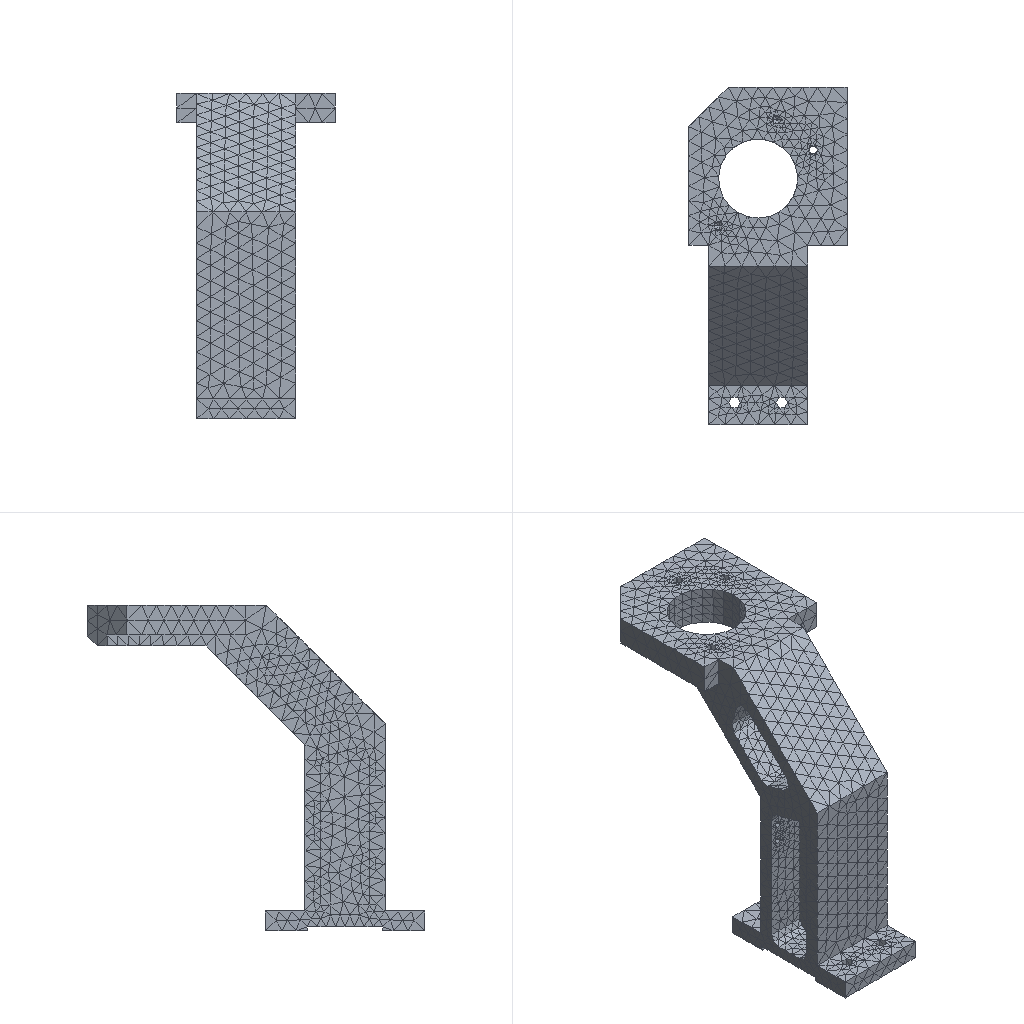Simulation study | nx simcenter
Set-up summary:
category,name,step,type,value,unit,region
solver,nx_nastran (Simcenter)
units,not stated in the deck,,not stated
analysis,deck,,static,static
analysis,solution,,SOL,101
load_step,SUBCASE 1,1,SUBCASE,SPC=1 LOAD=2
load_step,requested,,,1
mesh,nodes,,,17368
mesh,elements,,,9381
element_type,CTETRA,,solid,9381
load,nodal force total,,FX,0.0,model units
load,nodal force total,,FY,0.0,model units
load,nodal force total,,FZ,-999999.923,model units
load,load commands in deck,,count,589
bc,support commands in deck,,count,405
analysis,NX solution 0,,Structural,Linear Statics - Single Constraint
check,setup vs results,,match,every grid point's frame and coordinates and every element id; grid points of CTETRA elements
Nastran input file, long lists of numbers shortened:
$*$$$$$$$$$$$$$$$$$$$$$$$$$$$$$$$$$$$$$$$$$$$$$$$$$$$$$$$$$$$$$$$$$
$*
$*                    NX v10.0.0.24 TRANSLATOR
$*                    FOR NX NASTRAN VERSION 10.0
$ (33 more lines like these left out)
ASSIGN OUTPUT2='124_sim1-solution_1.op2' UNIT=12
$*
$*$$$$$$$$$$$$$$$$$$$$$$$$$$$$$$$$$$$
$*
$* EXECUTIVE CONTROL
$*
$*$$$$$$$$$$$$$$$$$$$$$$$$$$$$$$$$$$$
$*
ID,NASTRAN,124_sim1-solution_1
SOL 101
CEND
$*
$*$$$$$$$$$$$$$$$$$$$$$$$$$$$$$$$$$$$
$*
$* CASE CONTROL
$*
$*$$$$$$$$$$$$$$$$$$$$$$$$$$$$$$$$$$$
$*
TITLE = Solution 1
ECHO = NONE
SPC = 1
OUTPUT
BCRESULTS(TRACTION,FORCE,PLOT) = ALL
DISPLACEMENT(PLOT) = ALL
ESE(PLOT) = ALL
FORCE(PLOT,CORNER) = ALL
OLOAD(PLOT) = ALL
SPCFORCES(PLOT) = ALL
STRAIN(PLOT,FIBER,CORNER) = ALL
STRESS(PLOT,CORNER) = ALL
$*  NX Step: Subcase - Static Loads 1
SUBCASE 1
LABEL = Subcase - Static Loads 1
LOAD = 2
$*
$*$$$$$$$$$$$$$$$$$$$$$$$$$$$$$$$$$$$
$*
$* BULK DATA
$*
$*$$$$$$$$$$$$$$$$$$$$$$$$$$$$$$$$$$$
$*
BEGIN BULK
$*
$* PARAM CARDS
$*
PARAM      K6ROT100.0000
PARAM     OIBULK     YES
PARAM    OMACHPR     YES
PARAM       POST      -2
PARAM    POSTEXT     YES
PARAM    UNITSYS   MN-MM
$*
$* GRID CARDS
$*
GRID*              17223               0-3.500000000E+017.0500000000E+01+
*       1.4950000000E+02               0
GRID*              17224               0-3.500000000E+017.0500000000E+01+
*       1.6450000000E+02               0
$ (34732 more lines like these left out)
$*
$* ELEMENT CARDS
$*
$*  NX Mesh Collector: Solid(1)
$*  NX Mesh: 3d_mesh(1)
CTETRA         1       1       1       2       3       4     456     457+
+            458     459     460     461
CTETRA         2       1       1       5       6       7     462     463+
+            464     465     466     467
$ (18758 more lines like these left out)
$*
$* PROPERTY CARDS
$*
$*  NX Property: PSOLID1
PSOLID         1       1       0                           SMECH
$*
$* MATERIAL CARDS
$*
$*  NX Material: Aluminum_2014
MAT1           17.3119+7        0.3300002.7940-62.1355-5
MATT1          1       1               2               3
TABLEM1        1                                                        +
+        20.00007.3119+7 21.11007.3119+7 23.89007.3119+7 37.78007.3119+7+
+        51.67007.3119+7 65.56007.2429+7 79.44007.2429+7 93.33007.1739+7+
+       107.22007.1049+7121.11007.0359+7135.00006.9670+7148.89006.8980+7+
+       162.78006.8290+7176.67006.6910+7190.56006.6221+7204.44006.4841+7+
+       218.33006.3461+7232.22006.1392+7246.11006.0012+7260.00005.8633+7+
+       273.89005.7253+7287.78005.5184+7301.67005.3804+7315.56005.1735+7+
+       329.44004.9665+7343.33004.7596+7357.22004.6216+7371.11004.4147+7+
+           ENDT
TABLEM1        2                                                        +
+        20.00000.330000 21.11000.330000    ENDT
TABLEM1        3                                                        +
+        20.00002.1600-5 93.33002.2500-5107.22002.2662-5121.11002.2824-5+
+       135.00002.2968-5148.89002.3130-5162.78002.3274-5176.67002.3418-5+
+       190.56002.3544-5204.44002.3688-5218.33002.3814-5232.22002.3958-5+
+       246.11002.4066-5260.00002.4192-5273.89002.4300-5287.78002.4408-5+
+       301.67002.4498-5315.56002.4606-5329.44002.4696-5343.33002.4786-5+
+       357.22002.4876-5371.11002.4984-5385.00002.5110-5398.89002.5254-5+
+       412.78002.5398-5426.67002.5560-5    ENDT
$*
$* LOAD AND CONSTRAINT CARDS
$*
$*  NX Load and Constraint: Fixed(1)
SPC            1    9404  123456  0.0000
SPC            1    9405  123456  0.0000
SPC            1    9406  123456  0.0000
SPC            1    9407  123456  0.0000
$ (401 more lines like these left out)
$*  NX Load and Constraint: Force(1)
FORCE          2   14179       0 2231.35  0.0000  0.0000-1.00000
FORCE          2   14180       0 2166.76  0.0000  0.0000-1.00000
FORCE          2   14181       0 3293.26  0.0000  0.0000-1.00000
FORCE          2   14182       0 2396.51  0.0000  0.0000-1.00000
$ (585 more lines like these left out)
ENDDATA bb23f97d
Results summary:
result,analysis,,,static
result,last_loadstep,,,1
result,primary field,,,displacements
result,reaction total,,FX,-0.02859,model units
result,reaction total,,FY,0.1583,model units
result,reaction total,,FZ,1000000.312,model units
result,NX solution 0,,loadcases,1,mm